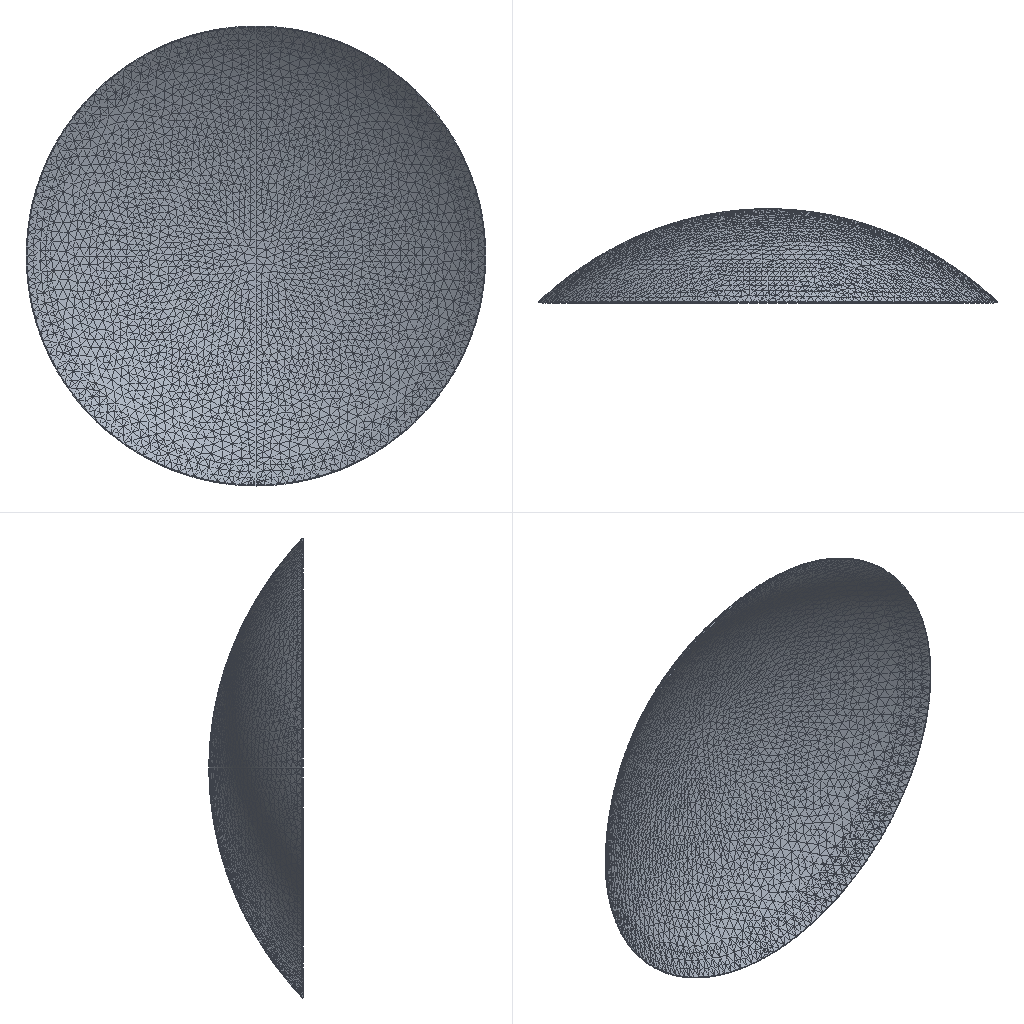Simulation study | abaqus
Set-up summary:
category,name,step,type,value,unit,region
solver,abaqus
solver,version,,,Abaqus/Explicit 2020
units,not stated in the deck,,not stated
analysis,deck,,transient,transient
load_step,Step-1,Step-1,transient
load_step,requested,,,1
mesh,nodes,,,12557
mesh,elements,,,26891
element_type,C3D4,,solid,21674
element_type,R3D3,,rigid,60
element_type,R3D4,,rigid,5157
load,load commands in deck,,count,1
bc,support commands in deck,,count,7
material,MATERIAL-1,,in results
check,setup vs results,,match,"per instance, exact: element labels, types and connectivity; labels of the nodes the elements use; coordinates of those nodes at SINGLE_PRECISION in 2 of 2 instance(s)"
Abaqus input file, long lists of numbers shortened:
*Heading
** Job name: Job-1 Model name: Model-1
** Generated by: Abaqus/CAE 2020
*Preprint, echo=NO, model=NO, history=NO, contact=NO
**
** PARTS
**
*Part, name=work-1
*Node
      1,           0.,  -1.075,  -3.913
      2,           0.,  -1.075,   3.913
** (5187 more lines like these left out)
*Element, type=R3D4
  1,    1,   25, 1263,  156
  2,   25,   26, 1264, 1263
** (5155 more lines like these left out)
*Element, type=R3D3
3037, 3244, 3245, 3661
3038, 3318, 3284, 3283
** (58 more lines like these left out)
*Node
   5190, 1.83637018e-15,  0.144,           0.
*Nset, nset=work-1-RefPt_, internal
5190,
*Elset, elset=work-1, generate
    1,  5217,     1
*End Part
**
*Part, name=work-2
*Node
      1,           0., -0.1298,           0.
      2,           0.,  -2.47,  -5.776
** (7365 more lines like these left out)
*Element, type=C3D4
    1, 6772,  876, 6775,  899
    2, 1434, 1460, 3976, 5321
** (21672 more lines like these left out)
*Nset, nset=Set-5, generate
    1,  7367,     1
*Elset, elset=Set-5, generate
     1,  21674,      1
** Section: Section-1
*Solid Section, elset=Set-5, material=Material-1
,
*End Part
**
**
** ASSEMBLY
**
*Assembly, name=Assembly
**
*Instance, name=work-1-1, part=work-1
*End Instance
**
*Instance, name=work-2-1, part=work-2
*End Instance
**
*Nset, nset=Set-1, instance=work-2-1
    2,    3,    4,    5,    6,    8,   42,   43,   44,   45,   46,   47,   48,   49,   50,   51
   52,   53,   54,   55,   56,   57,   58,   59,   60,   61,   62,   63,   64,   65,   66,   67
** (44 more lines like these left out)
*Elset, elset=Set-1, instance=work-2-1
   578,   664,   698,   779,   833,   883,   957,   959,  1027,  1096,  1104,  1360,  1387,  1420,  1485,  1521
  1635,  1701,  1707,  1709,  1755,  1756,  1776,  1866,  1879,  1884,  1895,  1974,  1975,  1976,  2040,  2052
** (58 more lines like these left out)
*Nset, nset=Set-2, instance=work-1-1
 5190,
*Elset, elset=_m_Surf-1_SPOS, internal, instance=work-1-1, generate
    1,  5217,     1
*Surface, type=ELEMENT, name=m_Surf-1
_m_Surf-1_SPOS, SPOS
*Elset, elset=_s_Surf-1_S2, internal, instance=work-2-1
     3,     8,     9,    16,    23,    29,    30,    33,    42,    46,    50,    53,    54,    56,    58,    61
    64,    65,    66,    70,    85,    93,    96,   100,   103,   107,   111,   112,   115,   116,   121,   125
** (225 more lines like these left out)
*Elset, elset=_s_Surf-1_S1, internal, instance=work-2-1
     4,     6,     7,    10,    12,    15,    18,    27,    37,    43,    48,    55,    57,    67,    69,    73
    77,    83,    86,   101,   106,   109,   110,   119,   122,   123,   124,   130,   132,   142,   145,   151
** (169 more lines like these left out)
*Elset, elset=_s_Surf-1_S4, internal, instance=work-2-1
    13,    14,    17,    20,    21,    24,    32,    36,    87,    90,   105,   118,   120,   128,   129,   135
   140,   149,   157,   162,   164,   172,   185,   187,   195,   206,   210,   229,   235,   245,   260,   261
** (160 more lines like these left out)
*Elset, elset=_s_Surf-1_S3, internal, instance=work-2-1
    28,    35,    38,    72,    76,    78,    79,    97,   102,   104,   113,   133,   200,   201,   234,   250
   251,   265,   274,   282,   293,   307,   358,   361,   369,   392,   419,   431,   433,   451,   464,   507
** (356 more lines like these left out)
*Surface, type=ELEMENT, name=s_Surf-1
_s_Surf-1_S2, S2
_s_Surf-1_S1, S1
_s_Surf-1_S4, S4
_s_Surf-1_S3, S3
*Rigid Body, ref node=work-1-1.work-1-RefPt_, elset=work-1-1.work-1
*End Assembly
*Amplitude, name=Amp-1
             0.,              0.,            0.01,              1.
**
** MATERIALS
**
*Material, name=Material-1
*Density
 1e-10,
*Elastic
1., 0.4
**
** INTERACTION PROPERTIES
**
*Surface Interaction, name=IntProp-1
*Friction
 0.2,
*Surface Behavior, pressure-overclosure=HARD
** ----------------------------------------------------------------
**
** STEP: Step-1
**
*Step, name=Step-1, nlgeom=YES
*Dynamic, Explicit
, 0.01
*Bulk Viscosity
0.06, 1.2
**
** BOUNDARY CONDITIONS
**
** Name: BC-1 Type: 对称/反对称/完全固定
*Boundary
Set-1, ENCASTRE
** Name: [REDACTED] : Displacement/rotation angle
*Boundary, amplitude=Amp-1
Set-2, 1, 1
Set-2, 2, 2, -0.5
Set-2, 3, 3
Set-2, 4, 4
Set-2, 5, 5
Set-2, 6, 6
**
** INTERACTIONS
**
** Interaction: Int-1
*Contact Pair, interaction=IntProp-1, mechanical constraint=KINEMATIC, cpset=Int-1
m_Surf-1, s_Surf-1
**
** OUTPUT REQUESTS
**
*Restart, write, number interval=1, time marks=NO
**
** FIELD OUTPUT: F-Output-1
**
*Output, field, number interval=50
*Node Output
A, CF, RF, RM, RT, U, V
*Element Output, directions=YES
E, EVF, LE, MISES, PE, PEEQ, PEEQVAVG, PEVAVG, S, SF, SSAVG, SVAVG
*Contact Output
CDISP, CSTRESS
**
** HISTORY OUTPUT: H-Output-1
**
*Output, history, variable=PRESELECT
*End Step
Results summary:
result,step,Step-1,partial,increments=93266 time=0.004265/0.01
result,analysis,,,transient
result,last_loadstep,,,1
result,primary field,,,U
result,reaction total,,FX,-1.9e-05,model units
result,reaction total,,FY,-0.000179,model units
result,reaction total,,FZ,2e-06,model units